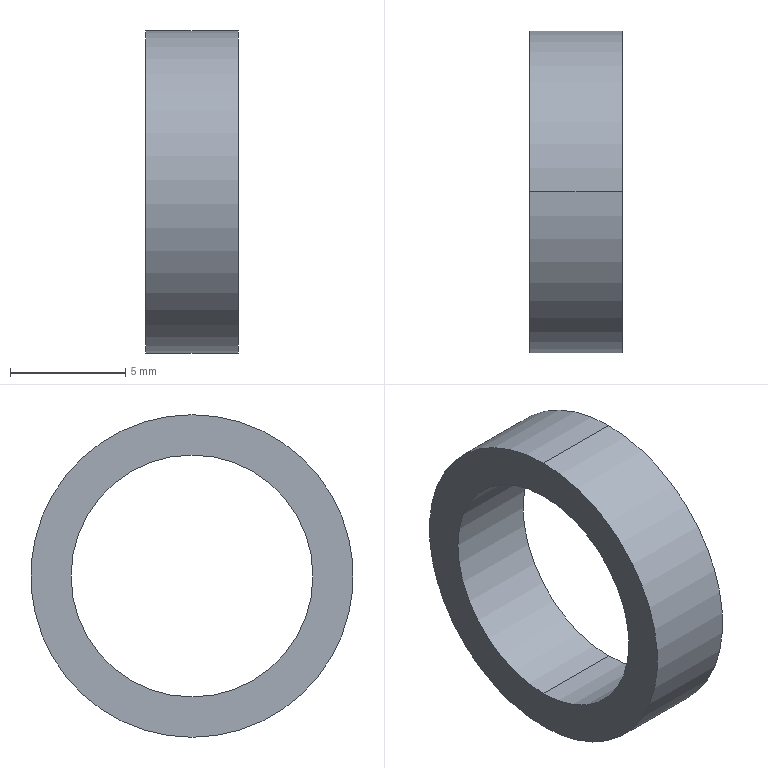Part | SolidWorks | features Extrusion 1 | 1 solid | 6 faces | box 4 x 14 x 14 mm | volume 269.392 mm3 | cylinder 4 | plane 2 | commonest cylinder face diameters 10.5 x2 14 x2
STEP:
#1=CARTESIAN_POINT('',(4.,0.,5.25));
#2=VERTEX_POINT('',#1);
#3=CARTESIAN_POINT('',(4.,0.,-5.25));
#4=VERTEX_POINT('',#3);
#5=CARTESIAN_POINT('',(4.,0.,0.));
#6=DIRECTION('',(1.,0.,0.));
#7=DIRECTION('',(0.,0.,-1.));
#8=AXIS2_PLACEMENT_3D('',#5,#6,#7);
#9=CIRCLE('',#8,5.25);
#10=EDGE_CURVE('',#2,#4,#9,.T.);
#11=ORIENTED_EDGE('',*,*,#10,.T.);
#12=CARTESIAN_POINT('',(0.,0.,-5.25));
#13=VERTEX_POINT('',#12);
#14=CARTESIAN_POINT('',(4.,0.,-5.25));
#15=DIRECTION('',(-1.,0.,0.));
#16=VECTOR('',#15,1000.);
#17=LINE('',#14,#16);
#18=EDGE_CURVE('',#4,#13,#17,.T.);
#19=ORIENTED_EDGE('',*,*,#18,.T.);
#20=CARTESIAN_POINT('',(0.,0.,5.25));
#21=VERTEX_POINT('',#20);
#22=CARTESIAN_POINT('',(0.,0.,0.));
#23=DIRECTION('',(1.,0.,0.));
#24=DIRECTION('',(0.,0.,-1.));
#25=AXIS2_PLACEMENT_3D('',#22,#23,#24);
#26=CIRCLE('',#25,5.25);
#27=EDGE_CURVE('',#21,#13,#26,.T.);
#28=ORIENTED_EDGE('',*,*,#27,.F.);
#29=CARTESIAN_POINT('',(4.,0.,5.25));
#30=DIRECTION('',(-1.,0.,0.));
#31=VECTOR('',#30,1000.);
#32=LINE('',#29,#31);
#33=EDGE_CURVE('',#2,#21,#32,.T.);
#34=ORIENTED_EDGE('',*,*,#33,.F.);
#35=EDGE_LOOP('',(#11,#19,#28,#34));
#36=FACE_OUTER_BOUND('',#35,.T.);
#37=CARTESIAN_POINT('',(4.,0.,0.));
#38=DIRECTION('',(-1.,0.,0.));
#39=DIRECTION('',(0.,0.,1.));
#40=AXIS2_PLACEMENT_3D('',#37,#38,#39);
#41=CYLINDRICAL_SURFACE('',#40,5.25);
#42=ADVANCED_FACE('',(#36),#41,.F.);
#43=CARTESIAN_POINT('',(4.,0.,-7.));
#44=VERTEX_POINT('',#43);
#45=CARTESIAN_POINT('',(4.,0.,7.));
#46=VERTEX_POINT('',#45);
#47=CARTESIAN_POINT('',(4.,0.,0.));
#48=DIRECTION('',(1.,0.,0.));
#49=DIRECTION('',(0.,0.,-1.));
#50=AXIS2_PLACEMENT_3D('',#47,#48,#49);
#51=CIRCLE('',#50,7.);
#52=EDGE_CURVE('',#44,#46,#51,.T.);
#53=ORIENTED_EDGE('',*,*,#52,.F.);
#54=CARTESIAN_POINT('',(0.,0.,-7.));
#55=VERTEX_POINT('',#54);
#56=CARTESIAN_POINT('',(4.,0.,-7.));
#57=DIRECTION('',(-1.,0.,0.));
#58=VECTOR('',#57,1000.);
#59=LINE('',#56,#58);
#60=EDGE_CURVE('',#44,#55,#59,.T.);
#61=ORIENTED_EDGE('',*,*,#60,.T.);
#62=CARTESIAN_POINT('',(0.,0.,7.));
#63=VERTEX_POINT('',#62);
#64=CARTESIAN_POINT('',(0.,0.,0.));
#65=DIRECTION('',(1.,0.,0.));
#66=DIRECTION('',(0.,0.,-1.));
#67=AXIS2_PLACEMENT_3D('',#64,#65,#66);
#68=CIRCLE('',#67,7.);
#69=EDGE_CURVE('',#55,#63,#68,.T.);
#70=ORIENTED_EDGE('',*,*,#69,.T.);
#71=CARTESIAN_POINT('',(4.,0.,7.));
#72=DIRECTION('',(-1.,0.,0.));
#73=VECTOR('',#72,1000.);
#74=LINE('',#71,#73);
#75=EDGE_CURVE('',#46,#63,#74,.T.);
#76=ORIENTED_EDGE('',*,*,#75,.F.);
#77=EDGE_LOOP('',(#53,#61,#70,#76));
#78=FACE_OUTER_BOUND('',#77,.T.);
#79=CARTESIAN_POINT('',(4.,0.,0.));
#80=DIRECTION('',(-1.,0.,0.));
#81=DIRECTION('',(0.,0.,1.));
#82=AXIS2_PLACEMENT_3D('',#79,#80,#81);
#83=CYLINDRICAL_SURFACE('',#82,7.);
#84=ADVANCED_FACE('',(#78),#83,.T.);
#85=CARTESIAN_POINT('',(4.,0.,0.));
#86=DIRECTION('',(1.,0.,0.));
#87=DIRECTION('',(0.,0.,-1.));
#88=AXIS2_PLACEMENT_3D('',#85,#86,#87);
#89=CIRCLE('',#88,7.);
#90=EDGE_CURVE('',#46,#44,#89,.T.);
#91=ORIENTED_EDGE('',*,*,#90,.T.);
#92=ORIENTED_EDGE('',*,*,#52,.T.);
#93=EDGE_LOOP('',(#91,#92));
#94=FACE_OUTER_BOUND('',#93,.T.);
#95=ORIENTED_EDGE('',*,*,#10,.F.);
#96=CARTESIAN_POINT('',(4.,0.,0.));
#97=DIRECTION('',(1.,0.,0.));
#98=DIRECTION('',(0.,0.,-1.));
#99=AXIS2_PLACEMENT_3D('',#96,#97,#98);
#100=CIRCLE('',#99,5.25);
#101=EDGE_CURVE('',#4,#2,#100,.T.);
#102=ORIENTED_EDGE('',*,*,#101,.F.);
#103=EDGE_LOOP('',(#95,#102));
#104=FACE_BOUND('',#103,.T.);
#105=CARTESIAN_POINT('',(4.,0.,0.));
#106=DIRECTION('',(1.,0.,0.));
#107=DIRECTION('',(0.,0.,-1.));
#108=AXIS2_PLACEMENT_3D('',#105,#106,#107);
#109=PLANE('',#108);
#110=ADVANCED_FACE('',(#94,#104),#109,.T.);
#111=CARTESIAN_POINT('',(0.,0.,0.));
#112=DIRECTION('',(1.,0.,0.));
#113=DIRECTION('',(0.,0.,-1.));
#114=AXIS2_PLACEMENT_3D('',#111,#112,#113);
#115=CIRCLE('',#114,7.);
#116=EDGE_CURVE('',#63,#55,#115,.T.);
#117=ORIENTED_EDGE('',*,*,#116,.F.);
#118=ORIENTED_EDGE('',*,*,#69,.F.);
#119=EDGE_LOOP('',(#117,#118));
#120=FACE_OUTER_BOUND('',#119,.T.);
#121=ORIENTED_EDGE('',*,*,#27,.T.);
#122=CARTESIAN_POINT('',(0.,0.,0.));
#123=DIRECTION('',(1.,0.,0.));
#124=DIRECTION('',(0.,0.,-1.));
#125=AXIS2_PLACEMENT_3D('',#122,#123,#124);
#126=CIRCLE('',#125,5.25);
#127=EDGE_CURVE('',#13,#21,#126,.T.);
#128=ORIENTED_EDGE('',*,*,#127,.T.);
#129=EDGE_LOOP('',(#121,#128));
#130=FACE_BOUND('',#129,.T.);
#131=CARTESIAN_POINT('',(0.,0.,0.));
#132=DIRECTION('',(1.,0.,0.));
#133=DIRECTION('',(0.,0.,-1.));
#134=AXIS2_PLACEMENT_3D('',#131,#132,#133);
#135=PLANE('',#134);
#136=ADVANCED_FACE('',(#120,#130),#135,.F.);
#137=ORIENTED_EDGE('',*,*,#60,.F.);
#138=ORIENTED_EDGE('',*,*,#90,.F.);
#139=ORIENTED_EDGE('',*,*,#75,.T.);
#140=ORIENTED_EDGE('',*,*,#116,.T.);
#141=EDGE_LOOP('',(#137,#138,#139,#140));
#142=FACE_OUTER_BOUND('',#141,.T.);
#143=CARTESIAN_POINT('',(4.,0.,0.));
#144=DIRECTION('',(-1.,0.,0.));
#145=DIRECTION('',(0.,0.,1.));
#146=AXIS2_PLACEMENT_3D('',#143,#144,#145);
#147=CYLINDRICAL_SURFACE('',#146,7.);
#148=ADVANCED_FACE('',(#142),#147,.T.);
#149=ORIENTED_EDGE('',*,*,#18,.F.);
#150=ORIENTED_EDGE('',*,*,#101,.T.);
#151=ORIENTED_EDGE('',*,*,#33,.T.);
#152=ORIENTED_EDGE('',*,*,#127,.F.);
#153=EDGE_LOOP('',(#149,#150,#151,#152));
#154=FACE_OUTER_BOUND('',#153,.T.);
#155=CARTESIAN_POINT('',(4.,0.,0.));
#156=DIRECTION('',(-1.,0.,0.));
#157=DIRECTION('',(0.,0.,1.));
#158=AXIS2_PLACEMENT_3D('',#155,#156,#157);
#159=CYLINDRICAL_SURFACE('',#158,5.25);
#160=ADVANCED_FACE('',(#154),#159,.F.);
#161=CLOSED_SHELL('',(#42,#84,#110,#136,#148,#160));
#162=MANIFOLD_SOLID_BREP('',#161);
#163=CARTESIAN_POINT('',(0.,0.,0.));
#164=DIRECTION('',(0.,0.,1.));
#165=DIRECTION('',(1.,0.,0.));
#166=AXIS2_PLACEMENT_3D('',#163,#164,#165);
#167=(LENGTH_UNIT()NAMED_UNIT(*)SI_UNIT(.MILLI.,.METRE.));
#168=UNCERTAINTY_MEASURE_WITH_UNIT(LENGTH_MEASURE(0.00001),#167,'','');
#169=(NAMED_UNIT(*)PLANE_ANGLE_UNIT()SI_UNIT($,.RADIAN.));
#170=(NAMED_UNIT(*)SI_UNIT($,.STERADIAN.)SOLID_ANGLE_UNIT());
#171=(GEOMETRIC_REPRESENTATION_CONTEXT(3)GLOBAL_UNCERTAINTY_ASSIGNED_CONTEXT((#168))GLOBAL_UNIT_ASSIGNED_CONTEXT((#167,#169,#170))REPRESENTATION_CONTEXT('',''));
#172=ADVANCED_BREP_SHAPE_REPRESENTATION('',(#162,#166),#171);